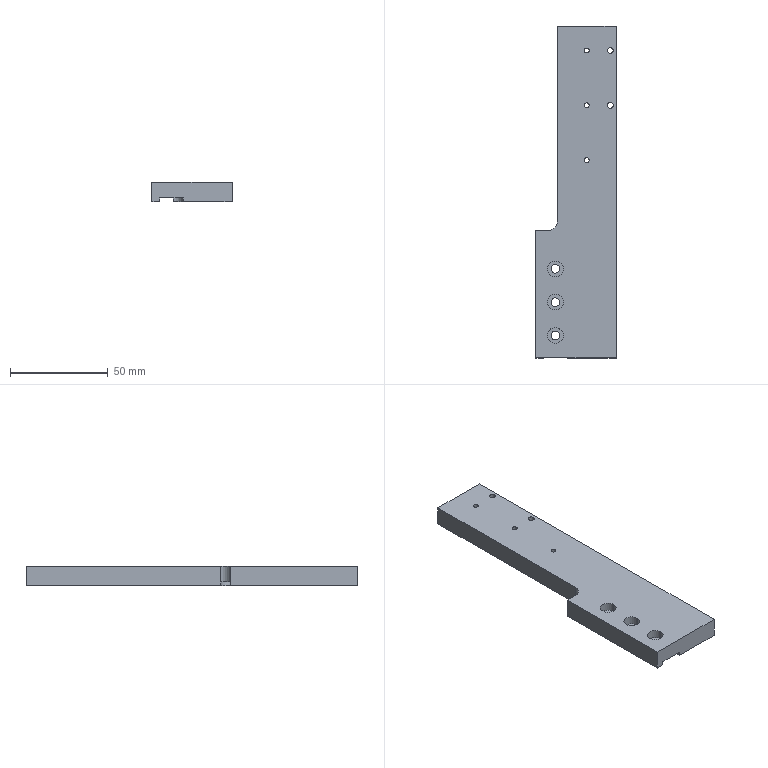Part | STEP file | 11-FG-E03311 | 1 solid | 39 faces | box 41 x 169.5 x 10 mm | volume 55320 mm3 | cylinder 24 | plane 15 | commonest cylinder face diameters 2.5 x6 4.5 x6 8 x6 3 x4 10 x2
STEP:
#1=CARTESIAN_POINT('',(-20.,-73.25,5.6));
#2=VERTEX_POINT('',#1);
#3=CARTESIAN_POINT('',(-12.,-73.25,5.6));
#4=VERTEX_POINT('',#3);
#5=CARTESIAN_POINT('',(-16.,-73.25,5.6));
#6=DIRECTION('',(0.,0.,1.));
#7=DIRECTION('',(1.,0.,0.));
#8=AXIS2_PLACEMENT_3D('',#5,#6,#7);
#9=CIRCLE('',#8,4.);
#10=EDGE_CURVE('',#2,#4,#9,.T.);
#11=ORIENTED_EDGE('',*,*,#10,.F.);
#12=CARTESIAN_POINT('',(-20.,-73.25,10.));
#13=VERTEX_POINT('',#12);
#14=CARTESIAN_POINT('',(-20.,-73.25,10.));
#15=DIRECTION('',(0.,0.,1.));
#16=VECTOR('',#15,1000.);
#17=LINE('',#14,#16);
#18=EDGE_CURVE('',#2,#13,#17,.T.);
#19=ORIENTED_EDGE('',*,*,#18,.T.);
#20=CARTESIAN_POINT('',(-12.,-73.25,10.));
#21=VERTEX_POINT('',#20);
#22=CARTESIAN_POINT('',(-16.,-73.25,10.));
#23=DIRECTION('',(0.,0.,1.));
#24=DIRECTION('',(1.,0.,0.));
#25=AXIS2_PLACEMENT_3D('',#22,#23,#24);
#26=CIRCLE('',#25,4.);
#27=EDGE_CURVE('',#13,#21,#26,.T.);
#28=ORIENTED_EDGE('',*,*,#27,.T.);
#29=CARTESIAN_POINT('',(-12.,-73.25,10.));
#30=DIRECTION('',(0.,0.,1.));
#31=VECTOR('',#30,1000.);
#32=LINE('',#29,#31);
#33=EDGE_CURVE('',#4,#21,#32,.T.);
#34=ORIENTED_EDGE('',*,*,#33,.F.);
#35=EDGE_LOOP('',(#11,#19,#28,#34));
#36=FACE_OUTER_BOUND('',#35,.T.);
#37=CARTESIAN_POINT('',(-16.,-73.25,10.));
#38=DIRECTION('',(0.,0.,1.));
#39=DIRECTION('',(1.,0.,0.));
#40=AXIS2_PLACEMENT_3D('',#37,#38,#39);
#41=CYLINDRICAL_SURFACE('',#40,4.);
#42=ADVANCED_FACE('',(#36),#41,.F.);
#43=CARTESIAN_POINT('',(-13.75,-73.25,2.));
#44=VERTEX_POINT('',#43);
#45=CARTESIAN_POINT('',(-18.25,-73.25,2.));
#46=VERTEX_POINT('',#45);
#47=CARTESIAN_POINT('',(-16.,-73.25,2.));
#48=DIRECTION('',(0.,0.,-1.));
#49=DIRECTION('',(-1.,0.,0.));
#50=AXIS2_PLACEMENT_3D('',#47,#48,#49);
#51=CIRCLE('',#50,2.25);
#52=EDGE_CURVE('',#44,#46,#51,.T.);
#53=ORIENTED_EDGE('',*,*,#52,.T.);
#54=CARTESIAN_POINT('',(-18.25,-73.25,5.6));
#55=VERTEX_POINT('',#54);
#56=CARTESIAN_POINT('',(-18.25,-73.25,10.));
#57=DIRECTION('',(0.,0.,1.));
#58=VECTOR('',#57,1000.);
#59=LINE('',#56,#58);
#60=EDGE_CURVE('',#46,#55,#59,.T.);
#61=ORIENTED_EDGE('',*,*,#60,.T.);
#62=CARTESIAN_POINT('',(-13.75,-73.25,5.6));
#63=VERTEX_POINT('',#62);
#64=CARTESIAN_POINT('',(-16.,-73.25,5.6));
#65=DIRECTION('',(0.,0.,1.));
#66=DIRECTION('',(1.,0.,0.));
#67=AXIS2_PLACEMENT_3D('',#64,#65,#66);
#68=CIRCLE('',#67,2.25);
#69=EDGE_CURVE('',#55,#63,#68,.T.);
#70=ORIENTED_EDGE('',*,*,#69,.T.);
#71=CARTESIAN_POINT('',(-13.75,-73.25,10.));
#72=DIRECTION('',(0.,0.,1.));
#73=VECTOR('',#72,1000.);
#74=LINE('',#71,#73);
#75=EDGE_CURVE('',#44,#63,#74,.T.);
#76=ORIENTED_EDGE('',*,*,#75,.F.);
#77=EDGE_LOOP('',(#53,#61,#70,#76));
#78=FACE_OUTER_BOUND('',#77,.T.);
#79=CARTESIAN_POINT('',(-16.,-73.25,10.));
#80=DIRECTION('',(0.,0.,1.));
#81=DIRECTION('',(1.,0.,0.));
#82=AXIS2_PLACEMENT_3D('',#79,#80,#81);
#83=CYLINDRICAL_SURFACE('',#82,2.25);
#84=ADVANCED_FACE('',(#78),#83,.F.);
#85=CARTESIAN_POINT('',(-20.,-56.25,5.6));
#86=VERTEX_POINT('',#85);
#87=CARTESIAN_POINT('',(-12.,-56.25,5.6));
#88=VERTEX_POINT('',#87);
#89=CARTESIAN_POINT('',(-16.,-56.25,5.6));
#90=DIRECTION('',(0.,0.,1.));
#91=DIRECTION('',(1.,0.,0.));
#92=AXIS2_PLACEMENT_3D('',#89,#90,#91);
#93=CIRCLE('',#92,4.);
#94=EDGE_CURVE('',#86,#88,#93,.T.);
#95=ORIENTED_EDGE('',*,*,#94,.F.);
#96=CARTESIAN_POINT('',(-20.,-56.25,10.));
#97=VERTEX_POINT('',#96);
#98=CARTESIAN_POINT('',(-20.,-56.25,10.));
#99=DIRECTION('',(0.,0.,1.));
#100=VECTOR('',#99,1000.);
#101=LINE('',#98,#100);
#102=EDGE_CURVE('',#86,#97,#101,.T.);
#103=ORIENTED_EDGE('',*,*,#102,.T.);
#104=CARTESIAN_POINT('',(-12.,-56.25,10.));
#105=VERTEX_POINT('',#104);
#106=CARTESIAN_POINT('',(-16.,-56.25,10.));
#107=DIRECTION('',(0.,0.,1.));
#108=DIRECTION('',(1.,0.,0.));
#109=AXIS2_PLACEMENT_3D('',#106,#107,#108);
#110=CIRCLE('',#109,4.);
#111=EDGE_CURVE('',#97,#105,#110,.T.);
#112=ORIENTED_EDGE('',*,*,#111,.T.);
#113=CARTESIAN_POINT('',(-12.,-56.25,10.));
#114=DIRECTION('',(0.,0.,1.));
#115=VECTOR('',#114,1000.);
#116=LINE('',#113,#115);
#117=EDGE_CURVE('',#88,#105,#116,.T.);
#118=ORIENTED_EDGE('',*,*,#117,.F.);
#119=EDGE_LOOP('',(#95,#103,#112,#118));
#120=FACE_OUTER_BOUND('',#119,.T.);
#121=CARTESIAN_POINT('',(-16.,-56.25,10.));
#122=DIRECTION('',(0.,0.,1.));
#123=DIRECTION('',(1.,0.,0.));
#124=AXIS2_PLACEMENT_3D('',#121,#122,#123);
#125=CYLINDRICAL_SURFACE('',#124,4.);
#126=ADVANCED_FACE('',(#120),#125,.F.);
#127=CARTESIAN_POINT('',(-13.75,-56.25,2.));
#128=VERTEX_POINT('',#127);
#129=CARTESIAN_POINT('',(-18.25,-56.25,2.));
#130=VERTEX_POINT('',#129);
#131=CARTESIAN_POINT('',(-16.,-56.25,2.));
#132=DIRECTION('',(0.,0.,-1.));
#133=DIRECTION('',(-1.,0.,0.));
#134=AXIS2_PLACEMENT_3D('',#131,#132,#133);
#135=CIRCLE('',#134,2.25);
#136=EDGE_CURVE('',#128,#130,#135,.T.);
#137=ORIENTED_EDGE('',*,*,#136,.T.);
#138=CARTESIAN_POINT('',(-18.25,-56.25,5.6));
#139=VERTEX_POINT('',#138);
#140=CARTESIAN_POINT('',(-18.25,-56.25,10.));
#141=DIRECTION('',(0.,0.,1.));
#142=VECTOR('',#141,1000.);
#143=LINE('',#140,#142);
#144=EDGE_CURVE('',#130,#139,#143,.T.);
#145=ORIENTED_EDGE('',*,*,#144,.T.);
#146=CARTESIAN_POINT('',(-13.75,-56.25,5.6));
#147=VERTEX_POINT('',#146);
#148=CARTESIAN_POINT('',(-16.,-56.25,5.6));
#149=DIRECTION('',(0.,0.,1.));
#150=DIRECTION('',(1.,0.,0.));
#151=AXIS2_PLACEMENT_3D('',#148,#149,#150);
#152=CIRCLE('',#151,2.25);
#153=EDGE_CURVE('',#139,#147,#152,.T.);
#154=ORIENTED_EDGE('',*,*,#153,.T.);
#155=CARTESIAN_POINT('',(-13.75,-56.25,10.));
#156=DIRECTION('',(0.,0.,1.));
#157=VECTOR('',#156,1000.);
#158=LINE('',#155,#157);
#159=EDGE_CURVE('',#128,#147,#158,.T.);
#160=ORIENTED_EDGE('',*,*,#159,.F.);
#161=EDGE_LOOP('',(#137,#145,#154,#160));
#162=FACE_OUTER_BOUND('',#161,.T.);
#163=CARTESIAN_POINT('',(-16.,-56.25,10.));
#164=DIRECTION('',(0.,0.,1.));
#165=DIRECTION('',(1.,0.,0.));
#166=AXIS2_PLACEMENT_3D('',#163,#164,#165);
#167=CYLINDRICAL_SURFACE('',#166,2.25);
#168=ADVANCED_FACE('',(#162),#167,.F.);
#169=CARTESIAN_POINT('',(-20.,-39.25,5.6));
#170=VERTEX_POINT('',#169);
#171=CARTESIAN_POINT('',(-12.,-39.25,5.6));
#172=VERTEX_POINT('',#171);
#173=CARTESIAN_POINT('',(-16.,-39.25,5.6));
#174=DIRECTION('',(0.,0.,1.));
#175=DIRECTION('',(1.,0.,0.));
#176=AXIS2_PLACEMENT_3D('',#173,#174,#175);
#177=CIRCLE('',#176,4.);
#178=EDGE_CURVE('',#170,#172,#177,.T.);
#179=ORIENTED_EDGE('',*,*,#178,.F.);
#180=CARTESIAN_POINT('',(-20.,-39.25,10.));
#181=VERTEX_POINT('',#180);
#182=CARTESIAN_POINT('',(-20.,-39.25,10.));
#183=DIRECTION('',(0.,0.,1.));
#184=VECTOR('',#183,1000.);
#185=LINE('',#182,#184);
#186=EDGE_CURVE('',#170,#181,#185,.T.);
#187=ORIENTED_EDGE('',*,*,#186,.T.);
#188=CARTESIAN_POINT('',(-12.,-39.25,10.));
#189=VERTEX_POINT('',#188);
#190=CARTESIAN_POINT('',(-16.,-39.25,10.));
#191=DIRECTION('',(0.,0.,1.));
#192=DIRECTION('',(1.,0.,0.));
#193=AXIS2_PLACEMENT_3D('',#190,#191,#192);
#194=CIRCLE('',#193,4.);
#195=EDGE_CURVE('',#181,#189,#194,.T.);
#196=ORIENTED_EDGE('',*,*,#195,.T.);
#197=CARTESIAN_POINT('',(-12.,-39.25,10.));
#198=DIRECTION('',(0.,0.,1.));
#199=VECTOR('',#198,1000.);
#200=LINE('',#197,#199);
#201=EDGE_CURVE('',#172,#189,#200,.T.);
#202=ORIENTED_EDGE('',*,*,#201,.F.);
#203=EDGE_LOOP('',(#179,#187,#196,#202));
#204=FACE_OUTER_BOUND('',#203,.T.);
#205=CARTESIAN_POINT('',(-16.,-39.25,10.));
#206=DIRECTION('',(0.,0.,1.));
#207=DIRECTION('',(1.,0.,0.));
#208=AXIS2_PLACEMENT_3D('',#205,#206,#207);
#209=CYLINDRICAL_SURFACE('',#208,4.);
#210=ADVANCED_FACE('',(#204),#209,.F.);
#211=CARTESIAN_POINT('',(-13.75,-39.25,2.));
#212=VERTEX_POINT('',#211);
#213=CARTESIAN_POINT('',(-18.25,-39.25,2.));
#214=VERTEX_POINT('',#213);
#215=CARTESIAN_POINT('',(-16.,-39.25,2.));
#216=DIRECTION('',(0.,0.,-1.));
#217=DIRECTION('',(-1.,0.,0.));
#218=AXIS2_PLACEMENT_3D('',#215,#216,#217);
#219=CIRCLE('',#218,2.25);
#220=EDGE_CURVE('',#212,#214,#219,.T.);
#221=ORIENTED_EDGE('',*,*,#220,.T.);
#222=CARTESIAN_POINT('',(-18.25,-39.25,5.6));
#223=VERTEX_POINT('',#222);
#224=CARTESIAN_POINT('',(-18.25,-39.25,10.));
#225=DIRECTION('',(0.,0.,1.));
#226=VECTOR('',#225,1000.);
#227=LINE('',#224,#226);
#228=EDGE_CURVE('',#214,#223,#227,.T.);
#229=ORIENTED_EDGE('',*,*,#228,.T.);
#230=CARTESIAN_POINT('',(-13.75,-39.25,5.6));
#231=VERTEX_POINT('',#230);
#232=CARTESIAN_POINT('',(-16.,-39.25,5.6));
#233=DIRECTION('',(0.,0.,1.));
#234=DIRECTION('',(1.,0.,0.));
#235=AXIS2_PLACEMENT_3D('',#232,#233,#234);
#236=CIRCLE('',#235,2.25);
#237=EDGE_CURVE('',#223,#231,#236,.T.);
#238=ORIENTED_EDGE('',*,*,#237,.T.);
#239=CARTESIAN_POINT('',(-13.75,-39.25,10.));
#240=DIRECTION('',(0.,0.,1.));
#241=VECTOR('',#240,1000.);
#242=LINE('',#239,#241);
#243=EDGE_CURVE('',#212,#231,#242,.T.);
#244=ORIENTED_EDGE('',*,*,#243,.F.);
#245=EDGE_LOOP('',(#221,#229,#238,#244));
#246=FACE_OUTER_BOUND('',#245,.T.);
#247=CARTESIAN_POINT('',(-16.,-39.25,10.));
#248=DIRECTION('',(0.,0.,1.));
#249=DIRECTION('',(1.,0.,0.));
#250=AXIS2_PLACEMENT_3D('',#247,#248,#249);
#251=CYLINDRICAL_SURFACE('',#250,2.25);
#252=ADVANCED_FACE('',(#246),#251,.F.);
#253=CARTESIAN_POINT('',(10.5,44.25,0.));
#254=VERTEX_POINT('',#253);
#255=CARTESIAN_POINT('',(13.5,44.25,0.));
#256=VERTEX_POINT('',#255);
#257=CARTESIAN_POINT('',(12.,44.25,0.));
#258=DIRECTION('',(0.,0.,1.));
#259=DIRECTION('',(1.,0.,0.));
#260=AXIS2_PLACEMENT_3D('',#257,#258,#259);
#261=CIRCLE('',#260,1.5);
#262=EDGE_CURVE('',#254,#256,#261,.T.);
#263=ORIENTED_EDGE('',*,*,#262,.F.);
#264=CARTESIAN_POINT('',(10.5,44.25,10.));
#265=VERTEX_POINT('',#264);
#266=CARTESIAN_POINT('',(10.5,44.25,10.));
#267=DIRECTION('',(0.,0.,1.));
#268=VECTOR('',#267,1000.);
#269=LINE('',#266,#268);
#270=EDGE_CURVE('',#254,#265,#269,.T.);
#271=ORIENTED_EDGE('',*,*,#270,.T.);
#272=CARTESIAN_POINT('',(13.5,44.25,10.));
#273=VERTEX_POINT('',#272);
#274=CARTESIAN_POINT('',(12.,44.25,10.));
#275=DIRECTION('',(0.,0.,1.));
#276=DIRECTION('',(1.,0.,0.));
#277=AXIS2_PLACEMENT_3D('',#274,#275,#276);
#278=CIRCLE('',#277,1.5);
#279=EDGE_CURVE('',#265,#273,#278,.T.);
#280=ORIENTED_EDGE('',*,*,#279,.T.);
#281=CARTESIAN_POINT('',(13.5,44.25,10.));
#282=DIRECTION('',(0.,0.,1.));
#283=VECTOR('',#282,1000.);
#284=LINE('',#281,#283);
#285=EDGE_CURVE('',#256,#273,#284,.T.);
#286=ORIENTED_EDGE('',*,*,#285,.F.);
#287=EDGE_LOOP('',(#263,#271,#280,#286));
#288=FACE_OUTER_BOUND('',#287,.T.);
#289=CARTESIAN_POINT('',(12.,44.25,10.));
#290=DIRECTION('',(0.,0.,1.));
#291=DIRECTION('',(1.,0.,0.));
#292=AXIS2_PLACEMENT_3D('',#289,#290,#291);
#293=CYLINDRICAL_SURFACE('',#292,1.5);
#294=ADVANCED_FACE('',(#288),#293,.F.);
#295=CARTESIAN_POINT('',(10.5,72.25,0.));
#296=VERTEX_POINT('',#295);
#297=CARTESIAN_POINT('',(13.5,72.25,0.));
#298=VERTEX_POINT('',#297);
#299=CARTESIAN_POINT('',(12.,72.25,0.));
#300=DIRECTION('',(0.,0.,1.));
#301=DIRECTION('',(1.,0.,0.));
#302=AXIS2_PLACEMENT_3D('',#299,#300,#301);
#303=CIRCLE('',#302,1.5);
#304=EDGE_CURVE('',#296,#298,#303,.T.);
#305=ORIENTED_EDGE('',*,*,#304,.F.);
#306=CARTESIAN_POINT('',(10.5,72.25,10.));
#307=VERTEX_POINT('',#306);
#308=CARTESIAN_POINT('',(10.5,72.25,10.));
#309=DIRECTION('',(0.,0.,1.));
#310=VECTOR('',#309,1000.);
#311=LINE('',#308,#310);
#312=EDGE_CURVE('',#296,#307,#311,.T.);
#313=ORIENTED_EDGE('',*,*,#312,.T.);
#314=CARTESIAN_POINT('',(13.5,72.25,10.));
#315=VERTEX_POINT('',#314);
#316=CARTESIAN_POINT('',(12.,72.25,10.));
#317=DIRECTION('',(0.,0.,1.));
#318=DIRECTION('',(1.,0.,0.));
#319=AXIS2_PLACEMENT_3D('',#316,#317,#318);
#320=CIRCLE('',#319,1.5);
#321=EDGE_CURVE('',#307,#315,#320,.T.);
#322=ORIENTED_EDGE('',*,*,#321,.T.);
#323=CARTESIAN_POINT('',(13.5,72.25,10.));
#324=DIRECTION('',(0.,0.,1.));
#325=VECTOR('',#324,1000.);
#326=LINE('',#323,#325);
#327=EDGE_CURVE('',#298,#315,#326,.T.);
#328=ORIENTED_EDGE('',*,*,#327,.F.);
#329=EDGE_LOOP('',(#305,#313,#322,#328));
#330=FACE_OUTER_BOUND('',#329,.T.);
#331=CARTESIAN_POINT('',(12.,72.25,10.));
#332=DIRECTION('',(0.,0.,1.));
#333=DIRECTION('',(1.,0.,0.));
#334=AXIS2_PLACEMENT_3D('',#331,#332,#333);
#335=CYLINDRICAL_SURFACE('',#334,1.5);
#336=ADVANCED_FACE('',(#330),#335,.F.);
#337=CARTESIAN_POINT('',(-1.25,16.25,0.));
#338=VERTEX_POINT('',#337);
#339=CARTESIAN_POINT('',(1.25,16.25,0.));
#340=VERTEX_POINT('',#339);
#341=CARTESIAN_POINT('',(0.,16.25,0.));
#342=DIRECTION('',(0.,0.,1.));
#343=DIRECTION('',(1.,0.,0.));
#344=AXIS2_PLACEMENT_3D('',#341,#342,#343);
#345=CIRCLE('',#344,1.25);
#346=EDGE_CURVE('',#338,#340,#345,.T.);
#347=ORIENTED_EDGE('',*,*,#346,.F.);
#348=CARTESIAN_POINT('',(-1.25,16.25,10.));
#349=VERTEX_POINT('',#348);
#350=CARTESIAN_POINT('',(-1.25,16.25,10.));
#351=DIRECTION('',(0.,0.,1.));
#352=VECTOR('',#351,1000.);
#353=LINE('',#350,#352);
#354=EDGE_CURVE('',#338,#349,#353,.T.);
#355=ORIENTED_EDGE('',*,*,#354,.T.);
#356=CARTESIAN_POINT('',(1.25,16.25,10.));
#357=VERTEX_POINT('',#356);
#358=CARTESIAN_POINT('',(0.,16.25,10.));
#359=DIRECTION('',(0.,0.,1.));
#360=DIRECTION('',(1.,0.,0.));
#361=AXIS2_PLACEMENT_3D('',#358,#359,#360);
#362=CIRCLE('',#361,1.25);
#363=EDGE_CURVE('',#349,#357,#362,.T.);
#364=ORIENTED_EDGE('',*,*,#363,.T.);
#365=CARTESIAN_POINT('',(1.25,16.25,10.));
#366=DIRECTION('',(0.,0.,1.));
#367=VECTOR('',#366,1000.);
#368=LINE('',#365,#367);
#369=EDGE_CURVE('',#340,#357,#368,.T.);
#370=ORIENTED_EDGE('',*,*,#369,.F.);
#371=EDGE_LOOP('',(#347,#355,#364,#370));
#372=FACE_OUTER_BOUND('',#371,.T.);
#373=CARTESIAN_POINT('',(0.,16.25,10.));
#374=DIRECTION('',(0.,0.,1.));
#375=DIRECTION('',(1.,0.,0.));
#376=AXIS2_PLACEMENT_3D('',#373,#374,#375);
#377=CYLINDRICAL_SURFACE('',#376,1.25);
#378=ADVANCED_FACE('',(#372),#377,.F.);
#379=CARTESIAN_POINT('',(-1.25,44.25,0.));
#380=VERTEX_POINT('',#379);
#381=CARTESIAN_POINT('',(1.25,44.25,0.));
#382=VERTEX_POINT('',#381);
#383=CARTESIAN_POINT('',(0.,44.25,0.));
#384=DIRECTION('',(0.,0.,1.));
#385=DIRECTION('',(1.,0.,0.));
#386=AXIS2_PLACEMENT_3D('',#383,#384,#385);
#387=CIRCLE('',#386,1.25);
#388=EDGE_CURVE('',#380,#382,#387,.T.);
#389=ORIENTED_EDGE('',*,*,#388,.F.);
#390=CARTESIAN_POINT('',(-1.25,44.25,10.));
#391=VERTEX_POINT('',#390);
#392=CARTESIAN_POINT('',(-1.25,44.25,10.));
#393=DIRECTION('',(0.,0.,1.));
#394=VECTOR('',#393,1000.);
#395=LINE('',#392,#394);
#396=EDGE_CURVE('',#380,#391,#395,.T.);
#397=ORIENTED_EDGE('',*,*,#396,.T.);
#398=CARTESIAN_POINT('',(1.25,44.25,10.));
#399=VERTEX_POINT('',#398);
#400=CARTESIAN_POINT('',(0.,44.25,10.));
#401=DIRECTION('',(0.,0.,1.));
#402=DIRECTION('',(1.,0.,0.));
#403=AXIS2_PLACEMENT_3D('',#400,#401,#402);
#404=CIRCLE('',#403,1.25);
#405=EDGE_CURVE('',#391,#399,#404,.T.);
#406=ORIENTED_EDGE('',*,*,#405,.T.);
#407=CARTESIAN_POINT('',(1.25,44.25,10.));
#408=DIRECTION('',(0.,0.,1.));
#409=VECTOR('',#408,1000.);
#410=LINE('',#407,#409);
#411=EDGE_CURVE('',#382,#399,#410,.T.);
#412=ORIENTED_EDGE('',*,*,#411,.F.);
#413=EDGE_LOOP('',(#389,#397,#406,#412));
#414=FACE_OUTER_BOUND('',#413,.T.);
#415=CARTESIAN_POINT('',(0.,44.25,10.));
#416=DIRECTION('',(0.,0.,1.));
#417=DIRECTION('',(1.,0.,0.));
#418=AXIS2_PLACEMENT_3D('',#415,#416,#417);
#419=CYLINDRICAL_SURFACE('',#418,1.25);
#420=ADVANCED_FACE('',(#414),#419,.F.);
#421=CARTESIAN_POINT('',(-1.25,72.25,0.));
#422=VERTEX_POINT('',#421);
#423=CARTESIAN_POINT('',(1.25,72.25,0.));
#424=VERTEX_POINT('',#423);
#425=CARTESIAN_POINT('',(0.,72.25,0.));
#426=DIRECTION('',(0.,0.,1.));
#427=DIRECTION('',(1.,0.,0.));
#428=AXIS2_PLACEMENT_3D('',#425,#426,#427);
#429=CIRCLE('',#428,1.25);
#430=EDGE_CURVE('',#422,#424,#429,.T.);
#431=ORIENTED_EDGE('',*,*,#430,.F.);
#432=CARTESIAN_POINT('',(-1.25,72.25,10.));
#433=VERTEX_POINT('',#432);
#434=CARTESIAN_POINT('',(-1.25,72.25,10.));
#435=DIRECTION('',(0.,0.,1.));
#436=VECTOR('',#435,1000.);
#437=LINE('',#434,#436);
#438=EDGE_CURVE('',#422,#433,#437,.T.);
#439=ORIENTED_EDGE('',*,*,#438,.T.);
#440=CARTESIAN_POINT('',(1.25,72.25,10.));
#441=VERTEX_POINT('',#440);
#442=CARTESIAN_POINT('',(0.,72.25,10.));
#443=DIRECTION('',(0.,0.,1.));
#444=DIRECTION('',(1.,0.,0.));
#445=AXIS2_PLACEMENT_3D('',#442,#443,#444);
#446=CIRCLE('',#445,1.25);
#447=EDGE_CURVE('',#433,#441,#446,.T.);
#448=ORIENTED_EDGE('',*,*,#447,.T.);
#449=CARTESIAN_POINT('',(1.25,72.25,10.));
#450=DIRECTION('',(0.,0.,1.));
#451=VECTOR('',#450,1000.);
#452=LINE('',#449,#451);
#453=EDGE_CURVE('',#424,#441,#452,.T.);
#454=ORIENTED_EDGE('',*,*,#453,.F.);
#455=EDGE_LOOP('',(#431,#439,#448,#454));
#456=FACE_OUTER_BOUND('',#455,.T.);
#457=CARTESIAN_POINT('',(0.,72.25,10.));
#458=DIRECTION('',(0.,0.,1.));
#459=DIRECTION('',(1.,0.,0.));
#460=AXIS2_PLACEMENT_3D('',#457,#458,#459);
#461=CYLINDRICAL_SURFACE('',#460,1.25);
#462=ADVANCED_FACE('',(#456),#461,.F.);
#463=CARTESIAN_POINT('',(-16.,-73.25,10.));
#464=DIRECTION('',(0.,0.,1.));
#465=DIRECTION('',(1.,0.,0.));
#466=AXIS2_PLACEMENT_3D('',#463,#464,#465);
#467=CIRCLE('',#466,4.);
#468=EDGE_CURVE('',#21,#13,#467,.T.);
#469=ORIENTED_EDGE('',*,*,#468,.F.);
#470=ORIENTED_EDGE('',*,*,#27,.F.);
#471=EDGE_LOOP('',(#469,#470));
#472=FACE_BOUND('',#471,.T.);
#473=CARTESIAN_POINT('',(-16.,-56.25,10.));
#474=DIRECTION('',(0.,0.,1.));
#475=DIRECTION('',(1.,0.,0.));
#476=AXIS2_PLACEMENT_3D('',#473,#474,#475);
#477=CIRCLE('',#476,4.);
#478=EDGE_CURVE('',#105,#97,#477,.T.);
#479=ORIENTED_EDGE('',*,*,#478,.F.);
#480=ORIENTED_EDGE('',*,*,#111,.F.);
#481=EDGE_LOOP('',(#479,#480));
#482=FACE_BOUND('',#481,.T.);
#483=CARTESIAN_POINT('',(12.,44.25,10.));
#484=DIRECTION('',(0.,0.,1.));
#485=DIRECTION('',(1.,0.,0.));
#486=AXIS2_PLACEMENT_3D('',#483,#484,#485);
#487=CIRCLE('',#486,1.5);
#488=EDGE_CURVE('',#273,#265,#487,.T.);
#489=ORIENTED_EDGE('',*,*,#488,.F.);
#490=ORIENTED_EDGE('',*,*,#279,.F.);
#491=EDGE_LOOP('',(#489,#490));
#492=FACE_BOUND('',#491,.T.);
#493=CARTESIAN_POINT('',(12.,72.25,10.));
#494=DIRECTION('',(0.,0.,1.));
#495=DIRECTION('',(1.,0.,0.));
#496=AXIS2_PLACEMENT_3D('',#493,#494,#495);
#497=CIRCLE('',#496,1.5);
#498=EDGE_CURVE('',#315,#307,#497,.T.);
#499=ORIENTED_EDGE('',*,*,#498,.F.);
#500=ORIENTED_EDGE('',*,*,#321,.F.);
#501=EDGE_LOOP('',(#499,#500));
#502=FACE_BOUND('',#501,.T.);
#503=CARTESIAN_POINT('',(0.,16.25,10.));
#504=DIRECTION('',(0.,0.,1.));
#505=DIRECTION('',(1.,0.,0.));
#506=AXIS2_PLACEMENT_3D('',#503,#504,#505);
#507=CIRCLE('',#506,1.25);
#508=EDGE_CURVE('',#357,#349,#507,.T.);
#509=ORIENTED_EDGE('',*,*,#508,.F.);
#510=ORIENTED_EDGE('',*,*,#363,.F.);
#511=EDGE_LOOP('',(#509,#510));
#512=FACE_BOUND('',#511,.T.);
#513=CARTESIAN_POINT('',(0.,44.25,10.));
#514=DIRECTION('',(0.,0.,1.));
#515=DIRECTION('',(1.,0.,0.));
#516=AXIS2_PLACEMENT_3D('',#513,#514,#515);
#517=CIRCLE('',#516,1.25);
#518=EDGE_CURVE('',#399,#391,#517,.T.);
#519=ORIENTED_EDGE('',*,*,#518,.F.);
#520=ORIENTED_EDGE('',*,*,#405,.F.);
#521=EDGE_LOOP('',(#519,#520));
#522=FACE_BOUND('',#521,.T.);
#523=CARTESIAN_POINT('',(0.,72.25,10.));
#524=DIRECTION('',(0.,0.,1.));
#525=DIRECTION('',(1.,0.,0.));
#526=AXIS2_PLACEMENT_3D('',#523,#524,#525);
#527=CIRCLE('',#526,1.25);
#528=EDGE_CURVE('',#441,#433,#527,.T.);
#529=ORIENTED_EDGE('',*,*,#528,.F.);
#530=ORIENTED_EDGE('',*,*,#447,.F.);
#531=EDGE_LOOP('',(#529,#530));
#532=FACE_BOUND('',#531,.T.);
#533=CARTESIAN_POINT('',(15.,-84.75,10.));
#534=VERTEX_POINT('',#533);
#535=CARTESIAN_POINT('',(15.,84.75,10.));
#536=VERTEX_POINT('',#535);
#537=CARTESIAN_POINT('',(15.,-84.75,10.));
#538=DIRECTION('',(0.,1.,0.));
#539=VECTOR('',#538,1000.);
#540=LINE('',#537,#539);
#541=EDGE_CURVE('',#534,#536,#540,.T.);
#542=ORIENTED_EDGE('',*,*,#541,.T.);
#543=CARTESIAN_POINT('',(-15.,84.75,10.));
#544=VERTEX_POINT('',#543);
#545=CARTESIAN_POINT('',(-15.,84.75,10.));
#546=DIRECTION('',(-1.,0.,0.));
#547=VECTOR('',#546,1000.);
#548=LINE('',#545,#547);
#549=EDGE_CURVE('',#536,#544,#548,.T.);
#550=ORIENTED_EDGE('',*,*,#549,.T.);
#551=CARTESIAN_POINT('',(-15.,-14.75,10.));
#552=VERTEX_POINT('',#551);
#553=CARTESIAN_POINT('',(-15.,-84.75,10.));
#554=DIRECTION('',(0.,-1.,0.));
#555=VECTOR('',#554,1000.);
#556=LINE('',#553,#555);
#557=EDGE_CURVE('',#544,#552,#556,.T.);
#558=ORIENTED_EDGE('',*,*,#557,.T.);
#559=CARTESIAN_POINT('',(-20.,-19.75,10.));
#560=VERTEX_POINT('',#559);
#561=CARTESIAN_POINT('',(-20.,-14.75,10.));
#562=DIRECTION('',(0.,0.,-1.));
#563=DIRECTION('',(-1.,0.,0.));
#564=AXIS2_PLACEMENT_3D('',#561,#562,#563);
#565=CIRCLE('',#564,5.);
#566=EDGE_CURVE('',#552,#560,#565,.T.);
#567=ORIENTED_EDGE('',*,*,#566,.T.);
#568=CARTESIAN_POINT('',(-26.,-19.75,10.));
#569=VERTEX_POINT('',#568);
#570=CARTESIAN_POINT('',(-15.,-19.75,10.));
#571=DIRECTION('',(-1.,0.,0.));
#572=VECTOR('',#571,1000.);
#573=LINE('',#570,#572);
#574=EDGE_CURVE('',#560,#569,#573,.T.);
#575=ORIENTED_EDGE('',*,*,#574,.T.);
#576=CARTESIAN_POINT('',(-26.,-84.75,10.));
#577=VERTEX_POINT('',#576);
#578=CARTESIAN_POINT('',(-26.,-84.75,10.));
#579=DIRECTION('',(0.,-1.,0.));
#580=VECTOR('',#579,1000.);
#581=LINE('',#578,#580);
#582=EDGE_CURVE('',#569,#577,#581,.T.);
#583=ORIENTED_EDGE('',*,*,#582,.T.);
#584=CARTESIAN_POINT('',(-15.,-84.75,10.));
#585=DIRECTION('',(1.,0.,0.));
#586=VECTOR('',#585,1000.);
#587=LINE('',#584,#586);
#588=EDGE_CURVE('',#577,#534,#587,.T.);
#589=ORIENTED_EDGE('',*,*,#588,.T.);
#590=EDGE_LOOP('',(#542,#550,#558,#567,#575,#583,#589));
#591=FACE_OUTER_BOUND('',#590,.T.);
#592=CARTESIAN_POINT('',(-16.,-39.25,10.));
#593=DIRECTION('',(0.,0.,1.));
#594=DIRECTION('',(1.,0.,0.));
#595=AXIS2_PLACEMENT_3D('',#592,#593,#594);
#596=CIRCLE('',#595,4.);
#597=EDGE_CURVE('',#189,#181,#596,.T.);
#598=ORIENTED_EDGE('',*,*,#597,.F.);
#599=ORIENTED_EDGE('',*,*,#195,.F.);
#600=EDGE_LOOP('',(#598,#599));
#601=FACE_BOUND('',#600,.T.);
#602=CARTESIAN_POINT('',(0.,0.,10.));
#603=DIRECTION('',(0.,0.,-1.));
#604=DIRECTION('',(-1.,0.,0.));
#605=AXIS2_PLACEMENT_3D('',#602,#603,#604);
#606=PLANE('',#605);
#607=ADVANCED_FACE('',(#472,#482,#492,#502,#512,#522,#532,#591,#601),#606,.F.);
#608=CARTESIAN_POINT('',(-22.,-84.75,0.));
#609=VERTEX_POINT('',#608);
#610=CARTESIAN_POINT('',(-22.,-19.75,0.));
#611=VERTEX_POINT('',#610);
#612=CARTESIAN_POINT('',(-22.,-84.75,0.));
#613=DIRECTION('',(0.,1.,0.));
#614=VECTOR('',#613,1000.);
#615=LINE('',#612,#614);
#616=EDGE_CURVE('',#609,#611,#615,.T.);
#617=ORIENTED_EDGE('',*,*,#616,.F.);
#618=CARTESIAN_POINT('',(-26.,-84.75,0.));
#619=VERTEX_POINT('',#618);
#620=CARTESIAN_POINT('',(-15.,-84.75,0.));
#621=DIRECTION('',(1.,0.,0.));
#622=VECTOR('',#621,1000.);
#623=LINE('',#620,#622);
#624=EDGE_CURVE('',#619,#609,#623,.T.);
#625=ORIENTED_EDGE('',*,*,#624,.F.);
#626=CARTESIAN_POINT('',(-26.,-19.75,0.));
#627=VERTEX_POINT('',#626);
#628=CARTESIAN_POINT('',(-26.,-84.75,0.));
#629=DIRECTION('',(0.,-1.,0.));
#630=VECTOR('',#629,1000.);
#631=LINE('',#628,#630);
#632=EDGE_CURVE('',#627,#619,#631,.T.);
#633=ORIENTED_EDGE('',*,*,#632,.F.);
#634=CARTESIAN_POINT('',(-15.,-19.75,0.));
#635=DIRECTION('',(-1.,0.,0.));
#636=VECTOR('',#635,1000.);
#637=LINE('',#634,#636);
#638=EDGE_CURVE('',#611,#627,#637,.T.);
#639=ORIENTED_EDGE('',*,*,#638,.F.);
#640=EDGE_LOOP('',(#617,#625,#633,#639));
#641=FACE_OUTER_BOUND('',#640,.T.);
#642=CARTESIAN_POINT('',(0.,0.,0.));
#643=DIRECTION('',(0.,0.,-1.));
#644=DIRECTION('',(-1.,0.,0.));
#645=AXIS2_PLACEMENT_3D('',#642,#643,#644);
#646=PLANE('',#645);
#647=ADVANCED_FACE('',(#641),#646,.T.);
#648=CARTESIAN_POINT('',(15.,-84.75,0.));
#649=VERTEX_POINT('',#648);
#650=CARTESIAN_POINT('',(15.,84.75,0.));
#651=VERTEX_POINT('',#650);
#652=CARTESIAN_POINT('',(15.,-84.75,0.));
#653=DIRECTION('',(0.,1.,0.));
#654=VECTOR('',#653,1000.);
#655=LINE('',#652,#654);
#656=EDGE_CURVE('',#649,#651,#655,.T.);
#657=ORIENTED_EDGE('',*,*,#656,.T.);
#658=CARTESIAN_POINT('',(15.,84.75,10.));
#659=DIRECTION('',(0.,0.,-1.));
#660=VECTOR('',#659,1000.);
#661=LINE('',#658,#660);
#662=EDGE_CURVE('',#536,#651,#661,.T.);
#663=ORIENTED_EDGE('',*,*,#662,.F.);
#664=ORIENTED_EDGE('',*,*,#541,.F.);
#665=CARTESIAN_POINT('',(15.,-84.75,10.));
#666=DIRECTION('',(0.,0.,-1.));
#667=VECTOR('',#666,1000.);
#668=LINE('',#665,#667);
#669=EDGE_CURVE('',#534,#649,#668,.T.);
#670=ORIENTED_EDGE('',*,*,#669,.T.);
#671=EDGE_LOOP('',(#657,#663,#664,#670));
#672=FACE_OUTER_BOUND('',#671,.T.);
#673=CARTESIAN_POINT('',(15.,-84.75,10.));
#674=DIRECTION('',(-1.,0.,0.));
#675=DIRECTION('',(0.,0.,1.));
#676=AXIS2_PLACEMENT_3D('',#673,#674,#675);
#677=PLANE('',#676);
#678=ADVANCED_FACE('',(#672),#677,.F.);
#679=CARTESIAN_POINT('',(-15.,84.75,0.));
#680=VERTEX_POINT('',#679);
#681=CARTESIAN_POINT('',(-15.,84.75,0.));
#682=DIRECTION('',(-1.,0.,0.));
#683=VECTOR('',#682,1000.);
#684=LINE('',#681,#683);
#685=EDGE_CURVE('',#651,#680,#684,.T.);
#686=ORIENTED_EDGE('',*,*,#685,.T.);
#687=CARTESIAN_POINT('',(-15.,84.75,10.));
#688=DIRECTION('',(0.,0.,-1.));
#689=VECTOR('',#688,1000.);
#690=LINE('',#687,#689);
#691=EDGE_CURVE('',#544,#680,#690,.T.);
#692=ORIENTED_EDGE('',*,*,#691,.F.);
#693=ORIENTED_EDGE('',*,*,#549,.F.);
#694=ORIENTED_EDGE('',*,*,#662,.T.);
#695=EDGE_LOOP('',(#686,#692,#693,#694));
#696=FACE_OUTER_BOUND('',#695,.T.);
#697=CARTESIAN_POINT('',(-15.,84.75,10.));
#698=DIRECTION('',(0.,-1.,0.));
#699=DIRECTION('',(0.,0.,-1.));
#700=AXIS2_PLACEMENT_3D('',#697,#698,#699);
#701=PLANE('',#700);
#702=ADVANCED_FACE('',(#696),#701,.F.);
#703=CARTESIAN_POINT('',(-15.,-14.75,0.));
#704=VERTEX_POINT('',#703);
#705=CARTESIAN_POINT('',(-15.,-14.75,2.));
#706=VERTEX_POINT('',#705);
#707=CARTESIAN_POINT('',(-15.,-14.75,10.));
#708=DIRECTION('',(0.,0.,1.));
#709=VECTOR('',#708,1000.);
#710=LINE('',#707,#709);
#711=EDGE_CURVE('',#704,#706,#710,.T.);
#712=ORIENTED_EDGE('',*,*,#711,.T.);
#713=CARTESIAN_POINT('',(-15.,-14.75,10.));
#714=DIRECTION('',(0.,0.,1.));
#715=VECTOR('',#714,1000.);
#716=LINE('',#713,#715);
#717=EDGE_CURVE('',#706,#552,#716,.T.);
#718=ORIENTED_EDGE('',*,*,#717,.T.);
#719=ORIENTED_EDGE('',*,*,#557,.F.);
#720=ORIENTED_EDGE('',*,*,#691,.T.);
#721=CARTESIAN_POINT('',(-15.,-84.75,0.));
#722=DIRECTION('',(0.,-1.,0.));
#723=VECTOR('',#722,1000.);
#724=LINE('',#721,#723);
#725=EDGE_CURVE('',#680,#704,#724,.T.);
#726=ORIENTED_EDGE('',*,*,#725,.T.);
#727=EDGE_LOOP('',(#712,#718,#719,#720,#726));
#728=FACE_OUTER_BOUND('',#727,.T.);
#729=CARTESIAN_POINT('',(-15.,-84.75,10.));
#730=DIRECTION('',(1.,0.,0.));
#731=DIRECTION('',(0.,0.,-1.));
#732=AXIS2_PLACEMENT_3D('',#729,#730,#731);
#733=PLANE('',#732);
#734=ADVANCED_FACE('',(#728),#733,.F.);
#735=ORIENTED_EDGE('',*,*,#624,.T.);
#736=CARTESIAN_POINT('',(-22.,-84.75,2.));
#737=VERTEX_POINT('',#736);
#738=CARTESIAN_POINT('',(-22.,-84.75,2.));
#739=DIRECTION('',(0.,0.,-1.));
#740=VECTOR('',#739,1000.);
#741=LINE('',#738,#740);
#742=EDGE_CURVE('',#737,#609,#741,.T.);
#743=ORIENTED_EDGE('',*,*,#742,.F.);
#744=CARTESIAN_POINT('',(-10.,-84.75,2.));
#745=VERTEX_POINT('',#744);
#746=CARTESIAN_POINT('',(-22.,-84.75,2.));
#747=DIRECTION('',(-1.,0.,0.));
#748=VECTOR('',#747,1000.);
#749=LINE('',#746,#748);
#750=EDGE_CURVE('',#745,#737,#749,.T.);
#751=ORIENTED_EDGE('',*,*,#750,.F.);
#752=CARTESIAN_POINT('',(-10.,-84.75,0.));
#753=VERTEX_POINT('',#752);
#754=CARTESIAN_POINT('',(-10.,-84.75,2.));
#755=DIRECTION('',(0.,0.,-1.));
#756=VECTOR('',#755,1000.);
#757=LINE('',#754,#756);
#758=EDGE_CURVE('',#745,#753,#757,.T.);
#759=ORIENTED_EDGE('',*,*,#758,.T.);
#760=CARTESIAN_POINT('',(-15.,-84.75,0.));
#761=DIRECTION('',(1.,0.,0.));
#762=VECTOR('',#761,1000.);
#763=LINE('',#760,#762);
#764=EDGE_CURVE('',#753,#649,#763,.T.);
#765=ORIENTED_EDGE('',*,*,#764,.T.);
#766=ORIENTED_EDGE('',*,*,#669,.F.);
#767=ORIENTED_EDGE('',*,*,#588,.F.);
#768=CARTESIAN_POINT('',(-26.,-84.75,-65.924));
#769=DIRECTION('',(0.,0.,1.));
#770=VECTOR('',#769,1000.);
#771=LINE('',#768,#770);
#772=EDGE_CURVE('',#619,#577,#771,.T.);
#773=ORIENTED_EDGE('',*,*,#772,.F.);
#774=EDGE_LOOP('',(#735,#743,#751,#759,#765,#766,#767,#773));
#775=FACE_OUTER_BOUND('',#774,.T.);
#776=CARTESIAN_POINT('',(-15.,-84.75,10.));
#777=DIRECTION('',(0.,1.,0.));
#778=DIRECTION('',(0.,0.,1.));
#779=AXIS2_PLACEMENT_3D('',#776,#777,#778);
#780=PLANE('',#779);
#781=ADVANCED_FACE('',(#775),#780,.F.);
#782=CARTESIAN_POINT('',(-10.,-19.75,0.));
#783=VERTEX_POINT('',#782);
#784=CARTESIAN_POINT('',(-10.,-84.75,0.));
#785=DIRECTION('',(0.,-1.,0.));
#786=VECTOR('',#785,1000.);
#787=LINE('',#784,#786);
#788=EDGE_CURVE('',#783,#753,#787,.T.);
#789=ORIENTED_EDGE('',*,*,#788,.F.);
#790=CARTESIAN_POINT('',(-15.,-19.75,0.));
#791=DIRECTION('',(0.,0.,1.));
#792=DIRECTION('',(-1.,0.,0.));
#793=AXIS2_PLACEMENT_3D('',#790,#791,#792);
#794=CIRCLE('',#793,5.);
#795=EDGE_CURVE('',#783,#704,#794,.T.);
#796=ORIENTED_EDGE('',*,*,#795,.T.);
#797=ORIENTED_EDGE('',*,*,#725,.F.);
#798=ORIENTED_EDGE('',*,*,#685,.F.);
#799=ORIENTED_EDGE('',*,*,#656,.F.);
#800=ORIENTED_EDGE('',*,*,#764,.F.);
#801=EDGE_LOOP('',(#789,#796,#797,#798,#799,#800));
#802=FACE_OUTER_BOUND('',#801,.T.);
#803=CARTESIAN_POINT('',(12.,44.25,0.));
#804=DIRECTION('',(0.,0.,1.));
#805=DIRECTION('',(1.,0.,0.));
#806=AXIS2_PLACEMENT_3D('',#803,#804,#805);
#807=CIRCLE('',#806,1.5);
#808=EDGE_CURVE('',#256,#254,#807,.T.);
#809=ORIENTED_EDGE('',*,*,#808,.T.);
#810=ORIENTED_EDGE('',*,*,#262,.T.);
#811=EDGE_LOOP('',(#809,#810));
#812=FACE_BOUND('',#811,.T.);
#813=CARTESIAN_POINT('',(12.,72.25,0.));
#814=DIRECTION('',(0.,0.,1.));
#815=DIRECTION('',(1.,0.,0.));
#816=AXIS2_PLACEMENT_3D('',#813,#814,#815);
#817=CIRCLE('',#816,1.5);
#818=EDGE_CURVE('',#298,#296,#817,.T.);
#819=ORIENTED_EDGE('',*,*,#818,.T.);
#820=ORIENTED_EDGE('',*,*,#304,.T.);
#821=EDGE_LOOP('',(#819,#820));
#822=FACE_BOUND('',#821,.T.);
#823=CARTESIAN_POINT('',(0.,16.25,0.));
#824=DIRECTION('',(0.,0.,1.));
#825=DIRECTION('',(1.,0.,0.));
#826=AXIS2_PLACEMENT_3D('',#823,#824,#825);
#827=CIRCLE('',#826,1.25);
#828=EDGE_CURVE('',#340,#338,#827,.T.);
#829=ORIENTED_EDGE('',*,*,#828,.T.);
#830=ORIENTED_EDGE('',*,*,#346,.T.);
#831=EDGE_LOOP('',(#829,#830));
#832=FACE_BOUND('',#831,.T.);
#833=CARTESIAN_POINT('',(0.,44.25,0.));
#834=DIRECTION('',(0.,0.,1.));
#835=DIRECTION('',(1.,0.,0.));
#836=AXIS2_PLACEMENT_3D('',#833,#834,#835);
#837=CIRCLE('',#836,1.25);
#838=EDGE_CURVE('',#382,#380,#837,.T.);
#839=ORIENTED_EDGE('',*,*,#838,.T.);
#840=ORIENTED_EDGE('',*,*,#388,.T.);
#841=EDGE_LOOP('',(#839,#840));
#842=FACE_BOUND('',#841,.T.);
#843=CARTESIAN_POINT('',(0.,72.25,0.));
#844=DIRECTION('',(0.,0.,1.));
#845=DIRECTION('',(1.,0.,0.));
#846=AXIS2_PLACEMENT_3D('',#843,#844,#845);
#847=CIRCLE('',#846,1.25);
#848=EDGE_CURVE('',#424,#422,#847,.T.);
#849=ORIENTED_EDGE('',*,*,#848,.T.);
#850=ORIENTED_EDGE('',*,*,#430,.T.);
#851=EDGE_LOOP('',(#849,#850));
#852=FACE_BOUND('',#851,.T.);
#853=CARTESIAN_POINT('',(0.,0.,0.));
#854=DIRECTION('',(0.,0.,-1.));
#855=DIRECTION('',(-1.,0.,0.));
#856=AXIS2_PLACEMENT_3D('',#853,#854,#855);
#857=PLANE('',#856);
#858=ADVANCED_FACE('',(#802,#812,#822,#832,#842,#852),#857,.T.);
#859=ORIENTED_EDGE('',*,*,#438,.F.);
#860=ORIENTED_EDGE('',*,*,#848,.F.);
#861=ORIENTED_EDGE('',*,*,#453,.T.);
#862=ORIENTED_EDGE('',*,*,#528,.T.);
#863=EDGE_LOOP('',(#859,#860,#861,#862));
#864=FACE_OUTER_BOUND('',#863,.T.);
#865=CARTESIAN_POINT('',(0.,72.25,10.));
#866=DIRECTION('',(0.,0.,1.));
#867=DIRECTION('',(1.,0.,0.));
#868=AXIS2_PLACEMENT_3D('',#865,#866,#867);
#869=CYLINDRICAL_SURFACE('',#868,1.25);
#870=ADVANCED_FACE('',(#864),#869,.F.);
#871=ORIENTED_EDGE('',*,*,#396,.F.);
#872=ORIENTED_EDGE('',*,*,#838,.F.);
#873=ORIENTED_EDGE('',*,*,#411,.T.);
#874=ORIENTED_EDGE('',*,*,#518,.T.);
#875=EDGE_LOOP('',(#871,#872,#873,#874));
#876=FACE_OUTER_BOUND('',#875,.T.);
#877=CARTESIAN_POINT('',(0.,44.25,10.));
#878=DIRECTION('',(0.,0.,1.));
#879=DIRECTION('',(1.,0.,0.));
#880=AXIS2_PLACEMENT_3D('',#877,#878,#879);
#881=CYLINDRICAL_SURFACE('',#880,1.25);
#882=ADVANCED_FACE('',(#876),#881,.F.);
#883=ORIENTED_EDGE('',*,*,#354,.F.);
#884=ORIENTED_EDGE('',*,*,#828,.F.);
#885=ORIENTED_EDGE('',*,*,#369,.T.);
#886=ORIENTED_EDGE('',*,*,#508,.T.);
#887=EDGE_LOOP('',(#883,#884,#885,#886));
#888=FACE_OUTER_BOUND('',#887,.T.);
#889=CARTESIAN_POINT('',(0.,16.25,10.));
#890=DIRECTION('',(0.,0.,1.));
#891=DIRECTION('',(1.,0.,0.));
#892=AXIS2_PLACEMENT_3D('',#889,#890,#891);
#893=CYLINDRICAL_SURFACE('',#892,1.25);
#894=ADVANCED_FACE('',(#888),#893,.F.);
#895=ORIENTED_EDGE('',*,*,#312,.F.);
#896=ORIENTED_EDGE('',*,*,#818,.F.);
#897=ORIENTED_EDGE('',*,*,#327,.T.);
#898=ORIENTED_EDGE('',*,*,#498,.T.);
#899=EDGE_LOOP('',(#895,#896,#897,#898));
#900=FACE_OUTER_BOUND('',#899,.T.);
#901=CARTESIAN_POINT('',(12.,72.25,10.));
#902=DIRECTION('',(0.,0.,1.));
#903=DIRECTION('',(1.,0.,0.));
#904=AXIS2_PLACEMENT_3D('',#901,#902,#903);
#905=CYLINDRICAL_SURFACE('',#904,1.5);
#906=ADVANCED_FACE('',(#900),#905,.F.);
#907=ORIENTED_EDGE('',*,*,#270,.F.);
#908=ORIENTED_EDGE('',*,*,#808,.F.);
#909=ORIENTED_EDGE('',*,*,#285,.T.);
#910=ORIENTED_EDGE('',*,*,#488,.T.);
#911=EDGE_LOOP('',(#907,#908,#909,#910));
#912=FACE_OUTER_BOUND('',#911,.T.);
#913=CARTESIAN_POINT('',(12.,44.25,10.));
#914=DIRECTION('',(0.,0.,1.));
#915=DIRECTION('',(1.,0.,0.));
#916=AXIS2_PLACEMENT_3D('',#913,#914,#915);
#917=CYLINDRICAL_SURFACE('',#916,1.5);
#918=ADVANCED_FACE('',(#912),#917,.F.);
#919=ORIENTED_EDGE('',*,*,#574,.F.);
#920=CARTESIAN_POINT('',(-20.,-19.75,2.));
#921=VERTEX_POINT('',#920);
#922=CARTESIAN_POINT('',(-20.,-19.75,-65.924));
#923=DIRECTION('',(0.,0.,-1.));
#924=VECTOR('',#923,1000.);
#925=LINE('',#922,#924);
#926=EDGE_CURVE('',#560,#921,#925,.T.);
#927=ORIENTED_EDGE('',*,*,#926,.T.);
#928=CARTESIAN_POINT('',(-22.,-19.75,2.));
#929=VERTEX_POINT('',#928);
#930=CARTESIAN_POINT('',(-15.,-19.75,2.));
#931=DIRECTION('',(-1.,0.,0.));
#932=VECTOR('',#931,1000.);
#933=LINE('',#930,#932);
#934=EDGE_CURVE('',#921,#929,#933,.T.);
#935=ORIENTED_EDGE('',*,*,#934,.T.);
#936=CARTESIAN_POINT('',(-22.,-19.75,-65.924));
#937=DIRECTION('',(0.,0.,1.));
#938=VECTOR('',#937,1000.);
#939=LINE('',#936,#938);
#940=EDGE_CURVE('',#611,#929,#939,.T.);
#941=ORIENTED_EDGE('',*,*,#940,.F.);
#942=ORIENTED_EDGE('',*,*,#638,.T.);
#943=CARTESIAN_POINT('',(-26.,-19.75,-65.924));
#944=DIRECTION('',(0.,0.,1.));
#945=VECTOR('',#944,1000.);
#946=LINE('',#943,#945);
#947=EDGE_CURVE('',#627,#569,#946,.T.);
#948=ORIENTED_EDGE('',*,*,#947,.T.);
#949=EDGE_LOOP('',(#919,#927,#935,#941,#942,#948));
#950=FACE_OUTER_BOUND('',#949,.T.);
#951=CARTESIAN_POINT('',(-15.,-19.75,-65.924));
#952=DIRECTION('',(0.,1.,0.));
#953=DIRECTION('',(0.,0.,1.));
#954=AXIS2_PLACEMENT_3D('',#951,#952,#953);
#955=PLANE('',#954);
#956=ADVANCED_FACE('',(#950),#955,.T.);
#957=ORIENTED_EDGE('',*,*,#947,.F.);
#958=ORIENTED_EDGE('',*,*,#632,.T.);
#959=ORIENTED_EDGE('',*,*,#772,.T.);
#960=ORIENTED_EDGE('',*,*,#582,.F.);
#961=EDGE_LOOP('',(#957,#958,#959,#960));
#962=FACE_OUTER_BOUND('',#961,.T.);
#963=CARTESIAN_POINT('',(-26.,-84.75,-65.924));
#964=DIRECTION('',(-1.,0.,0.));
#965=DIRECTION('',(0.,0.,1.));
#966=AXIS2_PLACEMENT_3D('',#963,#964,#965);
#967=PLANE('',#966);
#968=ADVANCED_FACE('',(#962),#967,.T.);
#969=ORIENTED_EDGE('',*,*,#52,.F.);
#970=CARTESIAN_POINT('',(-16.,-73.25,2.));
#971=DIRECTION('',(0.,0.,-1.));
#972=DIRECTION('',(-1.,0.,0.));
#973=AXIS2_PLACEMENT_3D('',#970,#971,#972);
#974=CIRCLE('',#973,2.25);
#975=EDGE_CURVE('',#46,#44,#974,.T.);
#976=ORIENTED_EDGE('',*,*,#975,.F.);
#977=EDGE_LOOP('',(#969,#976));
#978=FACE_BOUND('',#977,.T.);
#979=ORIENTED_EDGE('',*,*,#136,.F.);
#980=CARTESIAN_POINT('',(-16.,-56.25,2.));
#981=DIRECTION('',(0.,0.,-1.));
#982=DIRECTION('',(-1.,0.,0.));
#983=AXIS2_PLACEMENT_3D('',#980,#981,#982);
#984=CIRCLE('',#983,2.25);
#985=EDGE_CURVE('',#130,#128,#984,.T.);
#986=ORIENTED_EDGE('',*,*,#985,.F.);
#987=EDGE_LOOP('',(#979,#986));
#988=FACE_BOUND('',#987,.T.);
#989=ORIENTED_EDGE('',*,*,#220,.F.);
#990=CARTESIAN_POINT('',(-16.,-39.25,2.));
#991=DIRECTION('',(0.,0.,-1.));
#992=DIRECTION('',(-1.,0.,0.));
#993=AXIS2_PLACEMENT_3D('',#990,#991,#992);
#994=CIRCLE('',#993,2.25);
#995=EDGE_CURVE('',#214,#212,#994,.T.);
#996=ORIENTED_EDGE('',*,*,#995,.F.);
#997=EDGE_LOOP('',(#989,#996));
#998=FACE_BOUND('',#997,.T.);
#999=CARTESIAN_POINT('',(-20.,-14.75,2.));
#1000=DIRECTION('',(0.,0.,1.));
#1001=DIRECTION('',(-1.,0.,0.));
#1002=AXIS2_PLACEMENT_3D('',#999,#1000,#1001);
#1003=CIRCLE('',#1002,5.);
#1004=EDGE_CURVE('',#921,#706,#1003,.T.);
#1005=ORIENTED_EDGE('',*,*,#1004,.T.);
#1006=CARTESIAN_POINT('',(-10.,-19.75,2.));
#1007=VERTEX_POINT('',#1006);
#1008=CARTESIAN_POINT('',(-15.,-19.75,2.));
#1009=DIRECTION('',(0.,0.,-1.));
#1010=DIRECTION('',(-1.,0.,0.));
#1011=AXIS2_PLACEMENT_3D('',#1008,#1009,#1010);
#1012=CIRCLE('',#1011,5.);
#1013=EDGE_CURVE('',#706,#1007,#1012,.T.);
#1014=ORIENTED_EDGE('',*,*,#1013,.T.);
#1015=CARTESIAN_POINT('',(-10.,-84.75,2.));
#1016=DIRECTION('',(0.,-1.,0.));
#1017=VECTOR('',#1016,1000.);
#1018=LINE('',#1015,#1017);
#1019=EDGE_CURVE('',#1007,#745,#1018,.T.);
#1020=ORIENTED_EDGE('',*,*,#1019,.T.);
#1021=ORIENTED_EDGE('',*,*,#750,.T.);
#1022=CARTESIAN_POINT('',(-22.,-84.75,2.));
#1023=DIRECTION('',(0.,1.,0.));
#1024=VECTOR('',#1023,1000.);
#1025=LINE('',#1022,#1024);
#1026=EDGE_CURVE('',#737,#929,#1025,.T.);
#1027=ORIENTED_EDGE('',*,*,#1026,.T.);
#1028=ORIENTED_EDGE('',*,*,#934,.F.);
#1029=EDGE_LOOP('',(#1005,#1014,#1020,#1021,#1027,#1028));
#1030=FACE_OUTER_BOUND('',#1029,.T.);
#1031=CARTESIAN_POINT('',(0.,0.,2.));
#1032=DIRECTION('',(0.,0.,-1.));
#1033=DIRECTION('',(-1.,0.,0.));
#1034=AXIS2_PLACEMENT_3D('',#1031,#1032,#1033);
#1035=PLANE('',#1034);
#1036=ADVANCED_FACE('',(#978,#988,#998,#1030),#1035,.T.);
#1037=ORIENTED_EDGE('',*,*,#940,.T.);
#1038=ORIENTED_EDGE('',*,*,#1026,.F.);
#1039=ORIENTED_EDGE('',*,*,#742,.T.);
#1040=ORIENTED_EDGE('',*,*,#616,.T.);
#1041=EDGE_LOOP('',(#1037,#1038,#1039,#1040));
#1042=FACE_OUTER_BOUND('',#1041,.T.);
#1043=CARTESIAN_POINT('',(-22.,-84.75,2.));
#1044=DIRECTION('',(-1.,0.,0.));
#1045=DIRECTION('',(0.,0.,1.));
#1046=AXIS2_PLACEMENT_3D('',#1043,#1044,#1045);
#1047=PLANE('',#1046);
#1048=ADVANCED_FACE('',(#1042),#1047,.F.);
#1049=ORIENTED_EDGE('',*,*,#1019,.F.);
#1050=CARTESIAN_POINT('',(-10.,-19.75,0.));
#1051=DIRECTION('',(0.,0.,-1.));
#1052=VECTOR('',#1051,1000.);
#1053=LINE('',#1050,#1052);
#1054=EDGE_CURVE('',#1007,#783,#1053,.T.);
#1055=ORIENTED_EDGE('',*,*,#1054,.T.);
#1056=ORIENTED_EDGE('',*,*,#788,.T.);
#1057=ORIENTED_EDGE('',*,*,#758,.F.);
#1058=EDGE_LOOP('',(#1049,#1055,#1056,#1057));
#1059=FACE_OUTER_BOUND('',#1058,.T.);
#1060=CARTESIAN_POINT('',(-10.,-84.75,2.));
#1061=DIRECTION('',(1.,0.,0.));
#1062=DIRECTION('',(0.,0.,-1.));
#1063=AXIS2_PLACEMENT_3D('',#1060,#1061,#1062);
#1064=PLANE('',#1063);
#1065=ADVANCED_FACE('',(#1059),#1064,.F.);
#1066=ORIENTED_EDGE('',*,*,#1004,.F.);
#1067=ORIENTED_EDGE('',*,*,#926,.F.);
#1068=ORIENTED_EDGE('',*,*,#566,.F.);
#1069=ORIENTED_EDGE('',*,*,#717,.F.);
#1070=EDGE_LOOP('',(#1066,#1067,#1068,#1069));
#1071=FACE_OUTER_BOUND('',#1070,.T.);
#1072=CARTESIAN_POINT('',(-20.,-14.75,10.));
#1073=DIRECTION('',(0.,0.,1.));
#1074=DIRECTION('',(1.,0.,0.));
#1075=AXIS2_PLACEMENT_3D('',#1072,#1073,#1074);
#1076=CYLINDRICAL_SURFACE('',#1075,5.);
#1077=ADVANCED_FACE('',(#1071),#1076,.F.);
#1078=ORIENTED_EDGE('',*,*,#1013,.F.);
#1079=ORIENTED_EDGE('',*,*,#711,.F.);
#1080=ORIENTED_EDGE('',*,*,#795,.F.);
#1081=ORIENTED_EDGE('',*,*,#1054,.F.);
#1082=EDGE_LOOP('',(#1078,#1079,#1080,#1081));
#1083=FACE_OUTER_BOUND('',#1082,.T.);
#1084=CARTESIAN_POINT('',(-15.,-19.75,2.));
#1085=DIRECTION('',(0.,0.,1.));
#1086=DIRECTION('',(1.,0.,0.));
#1087=AXIS2_PLACEMENT_3D('',#1084,#1085,#1086);
#1088=CYLINDRICAL_SURFACE('',#1087,5.);
#1089=ADVANCED_FACE('',(#1083),#1088,.F.);
#1090=ORIENTED_EDGE('',*,*,#228,.F.);
#1091=ORIENTED_EDGE('',*,*,#995,.T.);
#1092=ORIENTED_EDGE('',*,*,#243,.T.);
#1093=CARTESIAN_POINT('',(-16.,-39.25,5.6));
#1094=DIRECTION('',(0.,0.,1.));
#1095=DIRECTION('',(1.,0.,0.));
#1096=AXIS2_PLACEMENT_3D('',#1093,#1094,#1095);
#1097=CIRCLE('',#1096,2.25);
#1098=EDGE_CURVE('',#231,#223,#1097,.T.);
#1099=ORIENTED_EDGE('',*,*,#1098,.T.);
#1100=EDGE_LOOP('',(#1090,#1091,#1092,#1099));
#1101=FACE_OUTER_BOUND('',#1100,.T.);
#1102=CARTESIAN_POINT('',(-16.,-39.25,10.));
#1103=DIRECTION('',(0.,0.,1.));
#1104=DIRECTION('',(1.,0.,0.));
#1105=AXIS2_PLACEMENT_3D('',#1102,#1103,#1104);
#1106=CYLINDRICAL_SURFACE('',#1105,2.25);
#1107=ADVANCED_FACE('',(#1101),#1106,.F.);
#1108=ORIENTED_EDGE('',*,*,#1098,.F.);
#1109=ORIENTED_EDGE('',*,*,#237,.F.);
#1110=EDGE_LOOP('',(#1108,#1109));
#1111=FACE_BOUND('',#1110,.T.);
#1112=CARTESIAN_POINT('',(-16.,-39.25,5.6));
#1113=DIRECTION('',(0.,0.,1.));
#1114=DIRECTION('',(1.,0.,0.));
#1115=AXIS2_PLACEMENT_3D('',#1112,#1113,#1114);
#1116=CIRCLE('',#1115,4.);
#1117=EDGE_CURVE('',#172,#170,#1116,.T.);
#1118=ORIENTED_EDGE('',*,*,#1117,.T.);
#1119=ORIENTED_EDGE('',*,*,#178,.T.);
#1120=EDGE_LOOP('',(#1118,#1119));
#1121=FACE_OUTER_BOUND('',#1120,.T.);
#1122=CARTESIAN_POINT('',(-13.75,-39.25,5.6));
#1123=DIRECTION('',(0.,0.,-1.));
#1124=DIRECTION('',(-1.,0.,0.));
#1125=AXIS2_PLACEMENT_3D('',#1122,#1123,#1124);
#1126=PLANE('',#1125);
#1127=ADVANCED_FACE('',(#1111,#1121),#1126,.F.);
#1128=ORIENTED_EDGE('',*,*,#186,.F.);
#1129=ORIENTED_EDGE('',*,*,#1117,.F.);
#1130=ORIENTED_EDGE('',*,*,#201,.T.);
#1131=ORIENTED_EDGE('',*,*,#597,.T.);
#1132=EDGE_LOOP('',(#1128,#1129,#1130,#1131));
#1133=FACE_OUTER_BOUND('',#1132,.T.);
#1134=CARTESIAN_POINT('',(-16.,-39.25,10.));
#1135=DIRECTION('',(0.,0.,1.));
#1136=DIRECTION('',(1.,0.,0.));
#1137=AXIS2_PLACEMENT_3D('',#1134,#1135,#1136);
#1138=CYLINDRICAL_SURFACE('',#1137,4.);
#1139=ADVANCED_FACE('',(#1133),#1138,.F.);
#1140=ORIENTED_EDGE('',*,*,#144,.F.);
#1141=ORIENTED_EDGE('',*,*,#985,.T.);
#1142=ORIENTED_EDGE('',*,*,#159,.T.);
#1143=CARTESIAN_POINT('',(-16.,-56.25,5.6));
#1144=DIRECTION('',(0.,0.,1.));
#1145=DIRECTION('',(1.,0.,0.));
#1146=AXIS2_PLACEMENT_3D('',#1143,#1144,#1145);
#1147=CIRCLE('',#1146,2.25);
#1148=EDGE_CURVE('',#147,#139,#1147,.T.);
#1149=ORIENTED_EDGE('',*,*,#1148,.T.);
#1150=EDGE_LOOP('',(#1140,#1141,#1142,#1149));
#1151=FACE_OUTER_BOUND('',#1150,.T.);
#1152=CARTESIAN_POINT('',(-16.,-56.25,10.));
#1153=DIRECTION('',(0.,0.,1.));
#1154=DIRECTION('',(1.,0.,0.));
#1155=AXIS2_PLACEMENT_3D('',#1152,#1153,#1154);
#1156=CYLINDRICAL_SURFACE('',#1155,2.25);
#1157=ADVANCED_FACE('',(#1151),#1156,.F.);
#1158=ORIENTED_EDGE('',*,*,#1148,.F.);
#1159=ORIENTED_EDGE('',*,*,#153,.F.);
#1160=EDGE_LOOP('',(#1158,#1159));
#1161=FACE_BOUND('',#1160,.T.);
#1162=CARTESIAN_POINT('',(-16.,-56.25,5.6));
#1163=DIRECTION('',(0.,0.,1.));
#1164=DIRECTION('',(1.,0.,0.));
#1165=AXIS2_PLACEMENT_3D('',#1162,#1163,#1164);
#1166=CIRCLE('',#1165,4.);
#1167=EDGE_CURVE('',#88,#86,#1166,.T.);
#1168=ORIENTED_EDGE('',*,*,#1167,.T.);
#1169=ORIENTED_EDGE('',*,*,#94,.T.);
#1170=EDGE_LOOP('',(#1168,#1169));
#1171=FACE_OUTER_BOUND('',#1170,.T.);
#1172=CARTESIAN_POINT('',(-13.75,-56.25,5.6));
#1173=DIRECTION('',(0.,0.,-1.));
#1174=DIRECTION('',(-1.,0.,0.));
#1175=AXIS2_PLACEMENT_3D('',#1172,#1173,#1174);
#1176=PLANE('',#1175);
#1177=ADVANCED_FACE('',(#1161,#1171),#1176,.F.);
#1178=ORIENTED_EDGE('',*,*,#102,.F.);
#1179=ORIENTED_EDGE('',*,*,#1167,.F.);
#1180=ORIENTED_EDGE('',*,*,#117,.T.);
#1181=ORIENTED_EDGE('',*,*,#478,.T.);
#1182=EDGE_LOOP('',(#1178,#1179,#1180,#1181));
#1183=FACE_OUTER_BOUND('',#1182,.T.);
#1184=CARTESIAN_POINT('',(-16.,-56.25,10.));
#1185=DIRECTION('',(0.,0.,1.));
#1186=DIRECTION('',(1.,0.,0.));
#1187=AXIS2_PLACEMENT_3D('',#1184,#1185,#1186);
#1188=CYLINDRICAL_SURFACE('',#1187,4.);
#1189=ADVANCED_FACE('',(#1183),#1188,.F.);
#1190=ORIENTED_EDGE('',*,*,#60,.F.);
#1191=ORIENTED_EDGE('',*,*,#975,.T.);
#1192=ORIENTED_EDGE('',*,*,#75,.T.);
#1193=CARTESIAN_POINT('',(-16.,-73.25,5.6));
#1194=DIRECTION('',(0.,0.,1.));
#1195=DIRECTION('',(1.,0.,0.));
#1196=AXIS2_PLACEMENT_3D('',#1193,#1194,#1195);
#1197=CIRCLE('',#1196,2.25);
#1198=EDGE_CURVE('',#63,#55,#1197,.T.);
#1199=ORIENTED_EDGE('',*,*,#1198,.T.);
#1200=EDGE_LOOP('',(#1190,#1191,#1192,#1199));
#1201=FACE_OUTER_BOUND('',#1200,.T.);
#1202=CARTESIAN_POINT('',(-16.,-73.25,10.));
#1203=DIRECTION('',(0.,0.,1.));
#1204=DIRECTION('',(1.,0.,0.));
#1205=AXIS2_PLACEMENT_3D('',#1202,#1203,#1204);
#1206=CYLINDRICAL_SURFACE('',#1205,2.25);
#1207=ADVANCED_FACE('',(#1201),#1206,.F.);
#1208=ORIENTED_EDGE('',*,*,#1198,.F.);
#1209=ORIENTED_EDGE('',*,*,#69,.F.);
#1210=EDGE_LOOP('',(#1208,#1209));
#1211=FACE_BOUND('',#1210,.T.);
#1212=CARTESIAN_POINT('',(-16.,-73.25,5.6));
#1213=DIRECTION('',(0.,0.,1.));
#1214=DIRECTION('',(1.,0.,0.));
#1215=AXIS2_PLACEMENT_3D('',#1212,#1213,#1214);
#1216=CIRCLE('',#1215,4.);
#1217=EDGE_CURVE('',#4,#2,#1216,.T.);
#1218=ORIENTED_EDGE('',*,*,#1217,.T.);
#1219=ORIENTED_EDGE('',*,*,#10,.T.);
#1220=EDGE_LOOP('',(#1218,#1219));
#1221=FACE_OUTER_BOUND('',#1220,.T.);
#1222=CARTESIAN_POINT('',(-13.75,-73.25,5.6));
#1223=DIRECTION('',(0.,0.,-1.));
#1224=DIRECTION('',(-1.,0.,0.));
#1225=AXIS2_PLACEMENT_3D('',#1222,#1223,#1224);
#1226=PLANE('',#1225);
#1227=ADVANCED_FACE('',(#1211,#1221),#1226,.F.);
#1228=ORIENTED_EDGE('',*,*,#18,.F.);
#1229=ORIENTED_EDGE('',*,*,#1217,.F.);
#1230=ORIENTED_EDGE('',*,*,#33,.T.);
#1231=ORIENTED_EDGE('',*,*,#468,.T.);
#1232=EDGE_LOOP('',(#1228,#1229,#1230,#1231));
#1233=FACE_OUTER_BOUND('',#1232,.T.);
#1234=CARTESIAN_POINT('',(-16.,-73.25,10.));
#1235=DIRECTION('',(0.,0.,1.));
#1236=DIRECTION('',(1.,0.,0.));
#1237=AXIS2_PLACEMENT_3D('',#1234,#1235,#1236);
#1238=CYLINDRICAL_SURFACE('',#1237,4.);
#1239=ADVANCED_FACE('',(#1233),#1238,.F.);
#1240=CLOSED_SHELL('',(#42,#84,#126,#168,#210,#252,#294,#336,#378,#420,#462,#607,#647,#678,#702,#734,#781,#858,#870,#882,#894,#906,#918,#956,#968,#1036,#1048,#1065,#1077,#1089,#1107,#1127,#1139,#1157,#1177,#1189,#1207,#1227,#1239));
#1241=MANIFOLD_SOLID_BREP('',#1240);
#1242=CARTESIAN_POINT('',(0.,0.,0.));
#1243=DIRECTION('',(0.,0.,1.));
#1244=DIRECTION('',(1.,0.,0.));
#1245=AXIS2_PLACEMENT_3D('',#1242,#1243,#1244);
#1246=(LENGTH_UNIT()NAMED_UNIT(*)SI_UNIT(.MILLI.,.METRE.));
#1247=UNCERTAINTY_MEASURE_WITH_UNIT(LENGTH_MEASURE(0.00001),#1246,'','');
#1248=(NAMED_UNIT(*)PLANE_ANGLE_UNIT()SI_UNIT($,.RADIAN.));
#1249=(NAMED_UNIT(*)SI_UNIT($,.STERADIAN.)SOLID_ANGLE_UNIT());
#1250=(GEOMETRIC_REPRESENTATION_CONTEXT(3)GLOBAL_UNCERTAINTY_ASSIGNED_CONTEXT((#1247))GLOBAL_UNIT_ASSIGNED_CONTEXT((#1246,#1248,#1249))REPRESENTATION_CONTEXT('',''));
#1251=ADVANCED_BREP_SHAPE_REPRESENTATION('',(#1241,#1245),#1250);